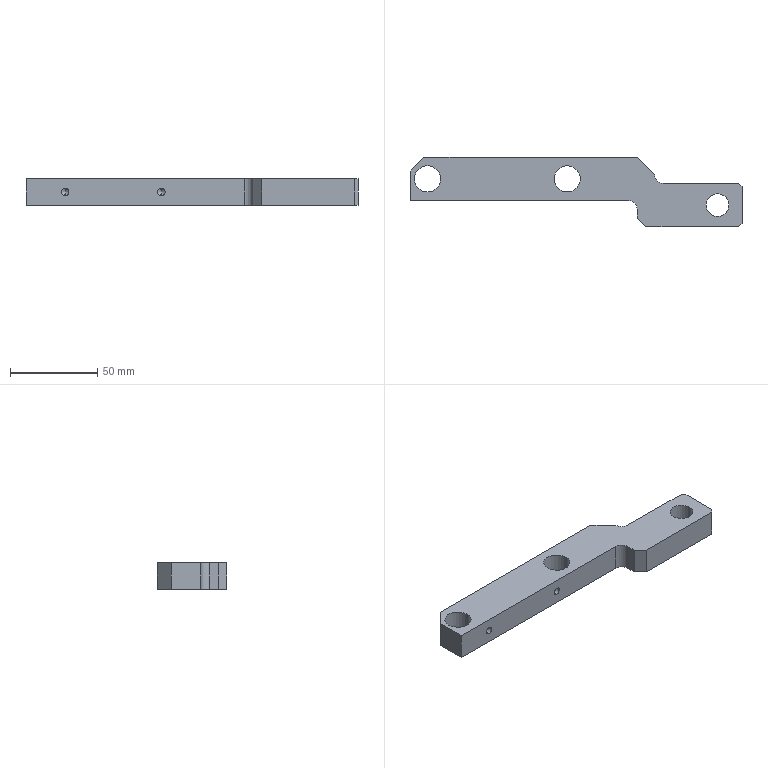Part | STEP file | CA-10-015Pusher Moving Plate2_Default | 1 solid | 33 faces | box 190 x 40 x 15.3 mm | volume 65560 mm3 | plane 15 | cylinder 14 | cone 4 | commonest cylinder face diameters 4.2 x4 15 x4 10 x2 13 x2 16 x2